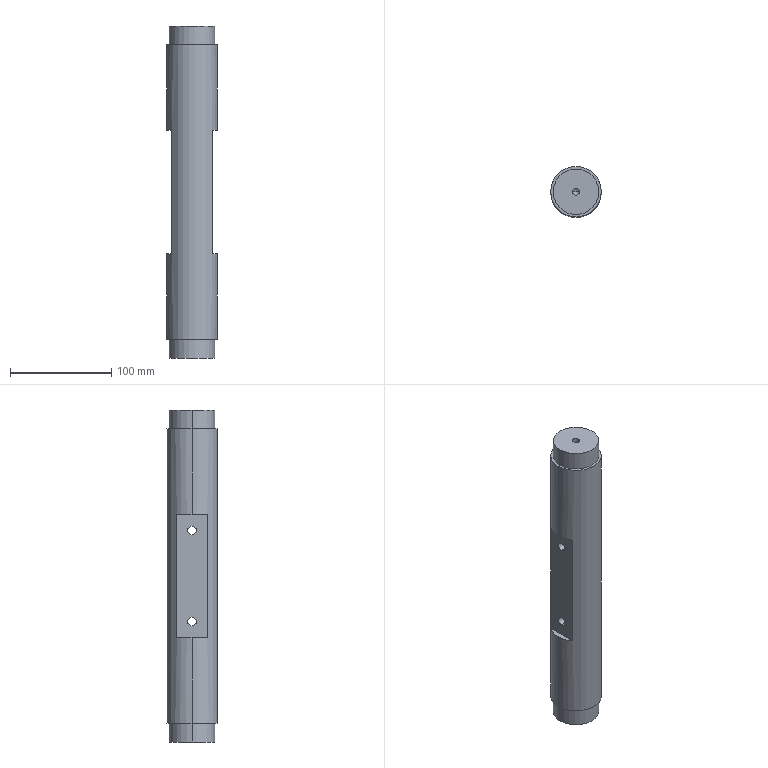Part | SolidWorks | features BaseBody 1 | 1 solid | 28 faces | box 50 x 50 x 328 mm | volume 599266 mm3 | cylinder 14 | plane 10 | cone 4 | commonest cylinder face diameters 6.8 x4 8.5 x4 45 x4 50 x2
STEP:
#1=CARTESIAN_POINT('',(-20.,0.,233.25));
#2=VERTEX_POINT('',#1);
#3=CARTESIAN_POINT('',(-20.,0.,224.75));
#4=VERTEX_POINT('',#3);
#5=CARTESIAN_POINT('',(-20.,0.,229.));
#6=DIRECTION('',(1.,0.,0.));
#7=DIRECTION('',(0.,0.,-1.));
#8=AXIS2_PLACEMENT_3D('',#5,#6,#7);
#9=CIRCLE('',#8,4.25);
#10=EDGE_CURVE('',#2,#4,#9,.T.);
#11=ORIENTED_EDGE('',*,*,#10,.F.);
#12=CARTESIAN_POINT('',(20.,0.,233.25));
#13=VERTEX_POINT('',#12);
#14=CARTESIAN_POINT('',(20.,0.,233.25));
#15=DIRECTION('',(1.,0.,0.));
#16=VECTOR('',#15,1000.);
#17=LINE('',#14,#16);
#18=EDGE_CURVE('',#2,#13,#17,.T.);
#19=ORIENTED_EDGE('',*,*,#18,.T.);
#20=CARTESIAN_POINT('',(20.,0.,224.75));
#21=VERTEX_POINT('',#20);
#22=CARTESIAN_POINT('',(20.,0.,229.));
#23=DIRECTION('',(1.,0.,0.));
#24=DIRECTION('',(0.,0.,-1.));
#25=AXIS2_PLACEMENT_3D('',#22,#23,#24);
#26=CIRCLE('',#25,4.25);
#27=EDGE_CURVE('',#13,#21,#26,.T.);
#28=ORIENTED_EDGE('',*,*,#27,.T.);
#29=CARTESIAN_POINT('',(20.,0.,224.75));
#30=DIRECTION('',(1.,0.,0.));
#31=VECTOR('',#30,1000.);
#32=LINE('',#29,#31);
#33=EDGE_CURVE('',#4,#21,#32,.T.);
#34=ORIENTED_EDGE('',*,*,#33,.F.);
#35=EDGE_LOOP('',(#11,#19,#28,#34));
#36=FACE_OUTER_BOUND('',#35,.T.);
#37=CARTESIAN_POINT('',(20.,0.,229.));
#38=DIRECTION('',(1.,0.,0.));
#39=DIRECTION('',(0.,0.,-1.));
#40=AXIS2_PLACEMENT_3D('',#37,#38,#39);
#41=CYLINDRICAL_SURFACE('',#40,4.25);
#42=ADVANCED_FACE('',(#36),#41,.F.);
#43=CARTESIAN_POINT('',(-20.,0.,143.25));
#44=VERTEX_POINT('',#43);
#45=CARTESIAN_POINT('',(-20.,0.,134.75));
#46=VERTEX_POINT('',#45);
#47=CARTESIAN_POINT('',(-20.,0.,139.));
#48=DIRECTION('',(1.,0.,0.));
#49=DIRECTION('',(0.,0.,-1.));
#50=AXIS2_PLACEMENT_3D('',#47,#48,#49);
#51=CIRCLE('',#50,4.25);
#52=EDGE_CURVE('',#44,#46,#51,.T.);
#53=ORIENTED_EDGE('',*,*,#52,.F.);
#54=CARTESIAN_POINT('',(20.,0.,143.25));
#55=VERTEX_POINT('',#54);
#56=CARTESIAN_POINT('',(20.,0.,143.25));
#57=DIRECTION('',(1.,0.,0.));
#58=VECTOR('',#57,1000.);
#59=LINE('',#56,#58);
#60=EDGE_CURVE('',#44,#55,#59,.T.);
#61=ORIENTED_EDGE('',*,*,#60,.T.);
#62=CARTESIAN_POINT('',(20.,0.,134.75));
#63=VERTEX_POINT('',#62);
#64=CARTESIAN_POINT('',(20.,0.,139.));
#65=DIRECTION('',(1.,0.,0.));
#66=DIRECTION('',(0.,0.,-1.));
#67=AXIS2_PLACEMENT_3D('',#64,#65,#66);
#68=CIRCLE('',#67,4.25);
#69=EDGE_CURVE('',#55,#63,#68,.T.);
#70=ORIENTED_EDGE('',*,*,#69,.T.);
#71=CARTESIAN_POINT('',(20.,0.,134.75));
#72=DIRECTION('',(1.,0.,0.));
#73=VECTOR('',#72,1000.);
#74=LINE('',#71,#73);
#75=EDGE_CURVE('',#46,#63,#74,.T.);
#76=ORIENTED_EDGE('',*,*,#75,.F.);
#77=EDGE_LOOP('',(#53,#61,#70,#76));
#78=FACE_OUTER_BOUND('',#77,.T.);
#79=CARTESIAN_POINT('',(20.,0.,139.));
#80=DIRECTION('',(1.,0.,0.));
#81=DIRECTION('',(0.,0.,-1.));
#82=AXIS2_PLACEMENT_3D('',#79,#80,#81);
#83=CYLINDRICAL_SURFACE('',#82,4.25);
#84=ADVANCED_FACE('',(#78),#83,.F.);
#85=CARTESIAN_POINT('',(3.4,0.,39.75));
#86=VERTEX_POINT('',#85);
#87=CARTESIAN_POINT('',(-3.4,0.,39.75));
#88=VERTEX_POINT('',#87);
#89=CARTESIAN_POINT('',(0.,0.,39.75));
#90=DIRECTION('',(0.,0.,-1.));
#91=DIRECTION('',(-1.,0.,0.));
#92=AXIS2_PLACEMENT_3D('',#89,#90,#91);
#93=CIRCLE('',#92,3.4);
#94=EDGE_CURVE('',#86,#88,#93,.T.);
#95=ORIENTED_EDGE('',*,*,#94,.F.);
#96=CARTESIAN_POINT('',(3.4,0.,20.));
#97=VERTEX_POINT('',#96);
#98=CARTESIAN_POINT('',(3.4,0.,20.));
#99=DIRECTION('',(0.,0.,-1.));
#100=VECTOR('',#99,1000.);
#101=LINE('',#98,#100);
#102=EDGE_CURVE('',#86,#97,#101,.T.);
#103=ORIENTED_EDGE('',*,*,#102,.T.);
#104=CARTESIAN_POINT('',(-3.4,0.,20.));
#105=VERTEX_POINT('',#104);
#106=CARTESIAN_POINT('',(0.,0.,20.));
#107=DIRECTION('',(0.,0.,-1.));
#108=DIRECTION('',(-1.,0.,0.));
#109=AXIS2_PLACEMENT_3D('',#106,#107,#108);
#110=CIRCLE('',#109,3.4);
#111=EDGE_CURVE('',#97,#105,#110,.T.);
#112=ORIENTED_EDGE('',*,*,#111,.T.);
#113=CARTESIAN_POINT('',(-3.4,0.,20.));
#114=DIRECTION('',(0.,0.,-1.));
#115=VECTOR('',#114,1000.);
#116=LINE('',#113,#115);
#117=EDGE_CURVE('',#88,#105,#116,.T.);
#118=ORIENTED_EDGE('',*,*,#117,.F.);
#119=EDGE_LOOP('',(#95,#103,#112,#118));
#120=FACE_OUTER_BOUND('',#119,.T.);
#121=CARTESIAN_POINT('',(0.,0.,20.));
#122=DIRECTION('',(0.,0.,-1.));
#123=DIRECTION('',(-1.,0.,0.));
#124=AXIS2_PLACEMENT_3D('',#121,#122,#123);
#125=CYLINDRICAL_SURFACE('',#124,3.4);
#126=ADVANCED_FACE('',(#120),#125,.F.);
#127=CARTESIAN_POINT('',(0.,0.,41.793));
#128=VERTEX_POINT('',#127);
#129=CARTESIAN_POINT('',(-3.4,0.,39.75));
#130=DIRECTION('',(-0.8572,0.,-0.515));
#131=VECTOR('',#130,1000.);
#132=LINE('',#129,#131);
#133=EDGE_CURVE('',#128,#88,#132,.T.);
#134=ORIENTED_EDGE('',*,*,#133,.F.);
#135=CARTESIAN_POINT('',(3.4,0.,39.75));
#136=DIRECTION('',(0.8572,0.,-0.515));
#137=VECTOR('',#136,1000.);
#138=LINE('',#135,#137);
#139=EDGE_CURVE('',#128,#86,#138,.T.);
#140=ORIENTED_EDGE('',*,*,#139,.T.);
#141=ORIENTED_EDGE('',*,*,#94,.T.);
#142=EDGE_LOOP('',(#134,#140,#141));
#143=FACE_OUTER_BOUND('',#142,.T.);
#144=CARTESIAN_POINT('',(0.,0.,39.75));
#145=DIRECTION('',(0.,0.,-1.));
#146=DIRECTION('',(-1.,0.,0.));
#147=AXIS2_PLACEMENT_3D('',#144,#145,#146);
#148=CONICAL_SURFACE('',#147,3.4,1.03);
#149=ADVANCED_FACE('',(#143),#148,.F.);
#150=CARTESIAN_POINT('',(-22.5,0.,38.5));
#151=VERTEX_POINT('',#150);
#152=CARTESIAN_POINT('',(22.5,0.,38.5));
#153=VERTEX_POINT('',#152);
#154=CARTESIAN_POINT('',(0.,0.,38.5));
#155=DIRECTION('',(0.,0.,-1.));
#156=DIRECTION('',(-1.,0.,0.));
#157=AXIS2_PLACEMENT_3D('',#154,#155,#156);
#158=CIRCLE('',#157,22.5);
#159=EDGE_CURVE('',#151,#153,#158,.T.);
#160=ORIENTED_EDGE('',*,*,#159,.T.);
#161=CARTESIAN_POINT('',(22.5,0.,20.));
#162=VERTEX_POINT('',#161);
#163=CARTESIAN_POINT('',(22.5,0.,38.5));
#164=DIRECTION('',(0.,0.,-1.));
#165=VECTOR('',#164,1000.);
#166=LINE('',#163,#165);
#167=EDGE_CURVE('',#153,#162,#166,.T.);
#168=ORIENTED_EDGE('',*,*,#167,.T.);
#169=CARTESIAN_POINT('',(-22.5,0.,20.));
#170=VERTEX_POINT('',#169);
#171=CARTESIAN_POINT('',(0.,0.,20.));
#172=DIRECTION('',(0.,0.,-1.));
#173=DIRECTION('',(-1.,0.,0.));
#174=AXIS2_PLACEMENT_3D('',#171,#172,#173);
#175=CIRCLE('',#174,22.5);
#176=EDGE_CURVE('',#170,#162,#175,.T.);
#177=ORIENTED_EDGE('',*,*,#176,.F.);
#178=CARTESIAN_POINT('',(-22.5,0.,38.5));
#179=DIRECTION('',(0.,0.,-1.));
#180=VECTOR('',#179,1000.);
#181=LINE('',#178,#180);
#182=EDGE_CURVE('',#151,#170,#181,.T.);
#183=ORIENTED_EDGE('',*,*,#182,.F.);
#184=EDGE_LOOP('',(#160,#168,#177,#183));
#185=FACE_OUTER_BOUND('',#184,.T.);
#186=CARTESIAN_POINT('',(0.,0.,38.5));
#187=DIRECTION('',(0.,0.,-1.));
#188=DIRECTION('',(-1.,0.,0.));
#189=AXIS2_PLACEMENT_3D('',#186,#187,#188);
#190=CYLINDRICAL_SURFACE('',#189,22.5);
#191=ADVANCED_FACE('',(#185),#190,.T.);
#192=CARTESIAN_POINT('',(-3.4,0.,328.25));
#193=VERTEX_POINT('',#192);
#194=CARTESIAN_POINT('',(3.4,0.,328.25));
#195=VERTEX_POINT('',#194);
#196=CARTESIAN_POINT('',(0.,0.,328.25));
#197=DIRECTION('',(0.,0.,1.));
#198=DIRECTION('',(1.,0.,0.));
#199=AXIS2_PLACEMENT_3D('',#196,#197,#198);
#200=CIRCLE('',#199,3.4);
#201=EDGE_CURVE('',#193,#195,#200,.T.);
#202=ORIENTED_EDGE('',*,*,#201,.F.);
#203=CARTESIAN_POINT('',(-3.4,0.,348.));
#204=VERTEX_POINT('',#203);
#205=CARTESIAN_POINT('',(-3.4,0.,348.));
#206=DIRECTION('',(0.,0.,1.));
#207=VECTOR('',#206,1000.);
#208=LINE('',#205,#207);
#209=EDGE_CURVE('',#193,#204,#208,.T.);
#210=ORIENTED_EDGE('',*,*,#209,.T.);
#211=CARTESIAN_POINT('',(3.4,0.,348.));
#212=VERTEX_POINT('',#211);
#213=CARTESIAN_POINT('',(0.,0.,348.));
#214=DIRECTION('',(0.,0.,1.));
#215=DIRECTION('',(1.,0.,0.));
#216=AXIS2_PLACEMENT_3D('',#213,#214,#215);
#217=CIRCLE('',#216,3.4);
#218=EDGE_CURVE('',#204,#212,#217,.T.);
#219=ORIENTED_EDGE('',*,*,#218,.T.);
#220=CARTESIAN_POINT('',(3.4,0.,348.));
#221=DIRECTION('',(0.,0.,1.));
#222=VECTOR('',#221,1000.);
#223=LINE('',#220,#222);
#224=EDGE_CURVE('',#195,#212,#223,.T.);
#225=ORIENTED_EDGE('',*,*,#224,.F.);
#226=EDGE_LOOP('',(#202,#210,#219,#225));
#227=FACE_OUTER_BOUND('',#226,.T.);
#228=CARTESIAN_POINT('',(0.,0.,348.));
#229=DIRECTION('',(0.,0.,1.));
#230=DIRECTION('',(1.,0.,0.));
#231=AXIS2_PLACEMENT_3D('',#228,#229,#230);
#232=CYLINDRICAL_SURFACE('',#231,3.4);
#233=ADVANCED_FACE('',(#227),#232,.F.);
#234=CARTESIAN_POINT('',(0.,0.,326.207));
#235=VERTEX_POINT('',#234);
#236=CARTESIAN_POINT('',(3.4,0.,328.25));
#237=DIRECTION('',(0.8572,0.,0.515));
#238=VECTOR('',#237,1000.);
#239=LINE('',#236,#238);
#240=EDGE_CURVE('',#235,#195,#239,.T.);
#241=ORIENTED_EDGE('',*,*,#240,.F.);
#242=CARTESIAN_POINT('',(-3.4,0.,328.25));
#243=DIRECTION('',(-0.8572,0.,0.515));
#244=VECTOR('',#243,1000.);
#245=LINE('',#242,#244);
#246=EDGE_CURVE('',#235,#193,#245,.T.);
#247=ORIENTED_EDGE('',*,*,#246,.T.);
#248=ORIENTED_EDGE('',*,*,#201,.T.);
#249=EDGE_LOOP('',(#241,#247,#248));
#250=FACE_OUTER_BOUND('',#249,.T.);
#251=CARTESIAN_POINT('',(0.,0.,328.25));
#252=DIRECTION('',(0.,0.,1.));
#253=DIRECTION('',(1.,0.,0.));
#254=AXIS2_PLACEMENT_3D('',#251,#252,#253);
#255=CONICAL_SURFACE('',#254,3.4,1.03);
#256=ADVANCED_FACE('',(#250),#255,.F.);
#257=CARTESIAN_POINT('',(22.5,0.,329.5));
#258=VERTEX_POINT('',#257);
#259=CARTESIAN_POINT('',(-22.5,0.,329.5));
#260=VERTEX_POINT('',#259);
#261=CARTESIAN_POINT('',(0.,0.,329.5));
#262=DIRECTION('',(0.,0.,1.));
#263=DIRECTION('',(1.,0.,0.));
#264=AXIS2_PLACEMENT_3D('',#261,#262,#263);
#265=CIRCLE('',#264,22.5);
#266=EDGE_CURVE('',#258,#260,#265,.T.);
#267=ORIENTED_EDGE('',*,*,#266,.T.);
#268=CARTESIAN_POINT('',(-22.5,0.,348.));
#269=VERTEX_POINT('',#268);
#270=CARTESIAN_POINT('',(-22.5,0.,329.5));
#271=DIRECTION('',(0.,0.,1.));
#272=VECTOR('',#271,1000.);
#273=LINE('',#270,#272);
#274=EDGE_CURVE('',#260,#269,#273,.T.);
#275=ORIENTED_EDGE('',*,*,#274,.T.);
#276=CARTESIAN_POINT('',(22.5,0.,348.));
#277=VERTEX_POINT('',#276);
#278=CARTESIAN_POINT('',(0.,0.,348.));
#279=DIRECTION('',(0.,0.,1.));
#280=DIRECTION('',(1.,0.,0.));
#281=AXIS2_PLACEMENT_3D('',#278,#279,#280);
#282=CIRCLE('',#281,22.5);
#283=EDGE_CURVE('',#277,#269,#282,.T.);
#284=ORIENTED_EDGE('',*,*,#283,.F.);
#285=CARTESIAN_POINT('',(22.5,0.,329.5));
#286=DIRECTION('',(0.,0.,1.));
#287=VECTOR('',#286,1000.);
#288=LINE('',#285,#287);
#289=EDGE_CURVE('',#258,#277,#288,.T.);
#290=ORIENTED_EDGE('',*,*,#289,.F.);
#291=EDGE_LOOP('',(#267,#275,#284,#290));
#292=FACE_OUTER_BOUND('',#291,.T.);
#293=CARTESIAN_POINT('',(0.,0.,329.5));
#294=DIRECTION('',(0.,0.,1.));
#295=DIRECTION('',(1.,0.,0.));
#296=AXIS2_PLACEMENT_3D('',#293,#294,#295);
#297=CYLINDRICAL_SURFACE('',#296,22.5);
#298=ADVANCED_FACE('',(#292),#297,.T.);
#299=CARTESIAN_POINT('',(25.,0.,329.5));
#300=VERTEX_POINT('',#299);
#301=CARTESIAN_POINT('',(-25.,0.,329.5));
#302=VERTEX_POINT('',#301);
#303=CARTESIAN_POINT('',(0.,0.,329.5));
#304=DIRECTION('',(0.,0.,1.));
#305=DIRECTION('',(1.,0.,0.));
#306=AXIS2_PLACEMENT_3D('',#303,#304,#305);
#307=CIRCLE('',#306,25.);
#308=EDGE_CURVE('',#300,#302,#307,.T.);
#309=ORIENTED_EDGE('',*,*,#308,.F.);
#310=CARTESIAN_POINT('',(25.,0.,245.));
#311=VERTEX_POINT('',#310);
#312=CARTESIAN_POINT('',(25.,0.,368.));
#313=DIRECTION('',(0.,0.,-1.));
#314=VECTOR('',#313,1000.);
#315=LINE('',#312,#314);
#316=EDGE_CURVE('',#300,#311,#315,.T.);
#317=ORIENTED_EDGE('',*,*,#316,.T.);
#318=CARTESIAN_POINT('',(20.,15.,245.));
#319=VERTEX_POINT('',#318);
#320=CARTESIAN_POINT('',(0.,0.,245.));
#321=DIRECTION('',(0.,0.,1.));
#322=DIRECTION('',(1.,0.,0.));
#323=AXIS2_PLACEMENT_3D('',#320,#321,#322);
#324=CIRCLE('',#323,25.);
#325=EDGE_CURVE('',#311,#319,#324,.T.);
#326=ORIENTED_EDGE('',*,*,#325,.T.);
#327=CARTESIAN_POINT('',(20.,15.,123.));
#328=VERTEX_POINT('',#327);
#329=CARTESIAN_POINT('',(20.,15.,368.));
#330=DIRECTION('',(0.,0.,-1.));
#331=VECTOR('',#330,1000.);
#332=LINE('',#329,#331);
#333=EDGE_CURVE('',#319,#328,#332,.T.);
#334=ORIENTED_EDGE('',*,*,#333,.T.);
#335=CARTESIAN_POINT('',(25.,0.,123.));
#336=VERTEX_POINT('',#335);
#337=CARTESIAN_POINT('',(0.,0.,123.));
#338=DIRECTION('',(0.,0.,-1.));
#339=DIRECTION('',(-1.,0.,0.));
#340=AXIS2_PLACEMENT_3D('',#337,#338,#339);
#341=CIRCLE('',#340,25.);
#342=EDGE_CURVE('',#328,#336,#341,.T.);
#343=ORIENTED_EDGE('',*,*,#342,.T.);
#344=CARTESIAN_POINT('',(25.,0.,38.5));
#345=VERTEX_POINT('',#344);
#346=CARTESIAN_POINT('',(25.,0.,368.));
#347=DIRECTION('',(0.,0.,-1.));
#348=VECTOR('',#347,1000.);
#349=LINE('',#346,#348);
#350=EDGE_CURVE('',#336,#345,#349,.T.);
#351=ORIENTED_EDGE('',*,*,#350,.T.);
#352=CARTESIAN_POINT('',(-25.,0.,38.5));
#353=VERTEX_POINT('',#352);
#354=CARTESIAN_POINT('',(0.,0.,38.5));
#355=DIRECTION('',(0.,0.,-1.));
#356=DIRECTION('',(-1.,0.,0.));
#357=AXIS2_PLACEMENT_3D('',#354,#355,#356);
#358=CIRCLE('',#357,25.);
#359=EDGE_CURVE('',#353,#345,#358,.T.);
#360=ORIENTED_EDGE('',*,*,#359,.F.);
#361=CARTESIAN_POINT('',(-25.,0.,123.));
#362=VERTEX_POINT('',#361);
#363=CARTESIAN_POINT('',(-25.,0.,368.));
#364=DIRECTION('',(0.,0.,-1.));
#365=VECTOR('',#364,1000.);
#366=LINE('',#363,#365);
#367=EDGE_CURVE('',#362,#353,#366,.T.);
#368=ORIENTED_EDGE('',*,*,#367,.F.);
#369=CARTESIAN_POINT('',(-20.,15.,123.));
#370=VERTEX_POINT('',#369);
#371=CARTESIAN_POINT('',(0.,0.,123.));
#372=DIRECTION('',(0.,0.,-1.));
#373=DIRECTION('',(-1.,0.,0.));
#374=AXIS2_PLACEMENT_3D('',#371,#372,#373);
#375=CIRCLE('',#374,25.);
#376=EDGE_CURVE('',#362,#370,#375,.T.);
#377=ORIENTED_EDGE('',*,*,#376,.T.);
#378=CARTESIAN_POINT('',(-20.,15.,245.));
#379=VERTEX_POINT('',#378);
#380=CARTESIAN_POINT('',(-20.,15.,368.));
#381=DIRECTION('',(0.,0.,1.));
#382=VECTOR('',#381,1000.);
#383=LINE('',#380,#382);
#384=EDGE_CURVE('',#370,#379,#383,.T.);
#385=ORIENTED_EDGE('',*,*,#384,.T.);
#386=CARTESIAN_POINT('',(-25.,0.,245.));
#387=VERTEX_POINT('',#386);
#388=CARTESIAN_POINT('',(0.,0.,245.));
#389=DIRECTION('',(0.,0.,1.));
#390=DIRECTION('',(1.,0.,0.));
#391=AXIS2_PLACEMENT_3D('',#388,#389,#390);
#392=CIRCLE('',#391,25.);
#393=EDGE_CURVE('',#379,#387,#392,.T.);
#394=ORIENTED_EDGE('',*,*,#393,.T.);
#395=CARTESIAN_POINT('',(-25.,0.,368.));
#396=DIRECTION('',(0.,0.,-1.));
#397=VECTOR('',#396,1000.);
#398=LINE('',#395,#397);
#399=EDGE_CURVE('',#302,#387,#398,.T.);
#400=ORIENTED_EDGE('',*,*,#399,.F.);
#401=EDGE_LOOP('',(#309,#317,#326,#334,#343,#351,#360,#368,#377,#385,#394,#400));
#402=FACE_OUTER_BOUND('',#401,.T.);
#403=CARTESIAN_POINT('',(0.,0.,368.));
#404=DIRECTION('',(0.,0.,-1.));
#405=DIRECTION('',(-1.,0.,0.));
#406=AXIS2_PLACEMENT_3D('',#403,#404,#405);
#407=CYLINDRICAL_SURFACE('',#406,25.);
#408=ADVANCED_FACE('',(#402),#407,.T.);
#409=CARTESIAN_POINT('',(20.,0.,229.));
#410=DIRECTION('',(1.,0.,0.));
#411=DIRECTION('',(0.,0.,-1.));
#412=AXIS2_PLACEMENT_3D('',#409,#410,#411);
#413=CIRCLE('',#412,4.25);
#414=EDGE_CURVE('',#21,#13,#413,.T.);
#415=ORIENTED_EDGE('',*,*,#414,.F.);
#416=ORIENTED_EDGE('',*,*,#27,.F.);
#417=EDGE_LOOP('',(#415,#416));
#418=FACE_BOUND('',#417,.T.);
#419=CARTESIAN_POINT('',(20.,-15.,245.));
#420=VERTEX_POINT('',#419);
#421=CARTESIAN_POINT('',(20.,-250.,245.));
#422=DIRECTION('',(0.,1.,0.));
#423=VECTOR('',#422,1000.);
#424=LINE('',#421,#423);
#425=EDGE_CURVE('',#420,#319,#424,.T.);
#426=ORIENTED_EDGE('',*,*,#425,.F.);
#427=CARTESIAN_POINT('',(20.,-15.,123.));
#428=VERTEX_POINT('',#427);
#429=CARTESIAN_POINT('',(20.,-15.,368.));
#430=DIRECTION('',(0.,0.,1.));
#431=VECTOR('',#430,1000.);
#432=LINE('',#429,#431);
#433=EDGE_CURVE('',#428,#420,#432,.T.);
#434=ORIENTED_EDGE('',*,*,#433,.F.);
#435=CARTESIAN_POINT('',(20.,-250.,123.));
#436=DIRECTION('',(0.,1.,0.));
#437=VECTOR('',#436,1000.);
#438=LINE('',#435,#437);
#439=EDGE_CURVE('',#428,#328,#438,.T.);
#440=ORIENTED_EDGE('',*,*,#439,.T.);
#441=ORIENTED_EDGE('',*,*,#333,.F.);
#442=EDGE_LOOP('',(#426,#434,#440,#441));
#443=FACE_OUTER_BOUND('',#442,.T.);
#444=CARTESIAN_POINT('',(20.,0.,139.));
#445=DIRECTION('',(1.,0.,0.));
#446=DIRECTION('',(0.,0.,-1.));
#447=AXIS2_PLACEMENT_3D('',#444,#445,#446);
#448=CIRCLE('',#447,4.25);
#449=EDGE_CURVE('',#63,#55,#448,.T.);
#450=ORIENTED_EDGE('',*,*,#449,.F.);
#451=ORIENTED_EDGE('',*,*,#69,.F.);
#452=EDGE_LOOP('',(#450,#451));
#453=FACE_BOUND('',#452,.T.);
#454=CARTESIAN_POINT('',(20.,-250.,123.));
#455=DIRECTION('',(-1.,0.,0.));
#456=DIRECTION('',(0.,0.,1.));
#457=AXIS2_PLACEMENT_3D('',#454,#455,#456);
#458=PLANE('',#457);
#459=ADVANCED_FACE('',(#418,#443,#453),#458,.F.);
#460=ORIENTED_EDGE('',*,*,#316,.F.);
#461=CARTESIAN_POINT('',(0.,0.,329.5));
#462=DIRECTION('',(0.,0.,1.));
#463=DIRECTION('',(1.,0.,0.));
#464=AXIS2_PLACEMENT_3D('',#461,#462,#463);
#465=CIRCLE('',#464,25.);
#466=EDGE_CURVE('',#302,#300,#465,.T.);
#467=ORIENTED_EDGE('',*,*,#466,.F.);
#468=ORIENTED_EDGE('',*,*,#399,.T.);
#469=CARTESIAN_POINT('',(-20.,-15.,245.));
#470=VERTEX_POINT('',#469);
#471=CARTESIAN_POINT('',(0.,0.,245.));
#472=DIRECTION('',(0.,0.,1.));
#473=DIRECTION('',(1.,0.,0.));
#474=AXIS2_PLACEMENT_3D('',#471,#472,#473);
#475=CIRCLE('',#474,25.);
#476=EDGE_CURVE('',#387,#470,#475,.T.);
#477=ORIENTED_EDGE('',*,*,#476,.T.);
#478=CARTESIAN_POINT('',(-20.,-15.,123.));
#479=VERTEX_POINT('',#478);
#480=CARTESIAN_POINT('',(-20.,-15.,368.));
#481=DIRECTION('',(0.,0.,-1.));
#482=VECTOR('',#481,1000.);
#483=LINE('',#480,#482);
#484=EDGE_CURVE('',#470,#479,#483,.T.);
#485=ORIENTED_EDGE('',*,*,#484,.T.);
#486=CARTESIAN_POINT('',(0.,0.,123.));
#487=DIRECTION('',(0.,0.,-1.));
#488=DIRECTION('',(-1.,0.,0.));
#489=AXIS2_PLACEMENT_3D('',#486,#487,#488);
#490=CIRCLE('',#489,25.);
#491=EDGE_CURVE('',#479,#362,#490,.T.);
#492=ORIENTED_EDGE('',*,*,#491,.T.);
#493=ORIENTED_EDGE('',*,*,#367,.T.);
#494=CARTESIAN_POINT('',(0.,0.,38.5));
#495=DIRECTION('',(0.,0.,-1.));
#496=DIRECTION('',(-1.,0.,0.));
#497=AXIS2_PLACEMENT_3D('',#494,#495,#496);
#498=CIRCLE('',#497,25.);
#499=EDGE_CURVE('',#345,#353,#498,.T.);
#500=ORIENTED_EDGE('',*,*,#499,.F.);
#501=ORIENTED_EDGE('',*,*,#350,.F.);
#502=CARTESIAN_POINT('',(0.,0.,123.));
#503=DIRECTION('',(0.,0.,-1.));
#504=DIRECTION('',(-1.,0.,0.));
#505=AXIS2_PLACEMENT_3D('',#502,#503,#504);
#506=CIRCLE('',#505,25.);
#507=EDGE_CURVE('',#336,#428,#506,.T.);
#508=ORIENTED_EDGE('',*,*,#507,.T.);
#509=ORIENTED_EDGE('',*,*,#433,.T.);
#510=CARTESIAN_POINT('',(0.,0.,245.));
#511=DIRECTION('',(0.,0.,1.));
#512=DIRECTION('',(1.,0.,0.));
#513=AXIS2_PLACEMENT_3D('',#510,#511,#512);
#514=CIRCLE('',#513,25.);
#515=EDGE_CURVE('',#420,#311,#514,.T.);
#516=ORIENTED_EDGE('',*,*,#515,.T.);
#517=EDGE_LOOP('',(#460,#467,#468,#477,#485,#492,#493,#500,#501,#508,#509,#516));
#518=FACE_OUTER_BOUND('',#517,.T.);
#519=CARTESIAN_POINT('',(0.,0.,368.));
#520=DIRECTION('',(0.,0.,-1.));
#521=DIRECTION('',(-1.,0.,0.));
#522=AXIS2_PLACEMENT_3D('',#519,#520,#521);
#523=CYLINDRICAL_SURFACE('',#522,25.);
#524=ADVANCED_FACE('',(#518),#523,.T.);
#525=ORIENTED_EDGE('',*,*,#439,.F.);
#526=ORIENTED_EDGE('',*,*,#507,.F.);
#527=ORIENTED_EDGE('',*,*,#342,.F.);
#528=EDGE_LOOP('',(#525,#526,#527));
#529=FACE_OUTER_BOUND('',#528,.T.);
#530=CARTESIAN_POINT('',(20.,-250.,123.));
#531=DIRECTION('',(0.,0.,-1.));
#532=DIRECTION('',(-1.,0.,0.));
#533=AXIS2_PLACEMENT_3D('',#530,#531,#532);
#534=PLANE('',#533);
#535=ADVANCED_FACE('',(#529),#534,.F.);
#536=ORIENTED_EDGE('',*,*,#425,.T.);
#537=ORIENTED_EDGE('',*,*,#325,.F.);
#538=ORIENTED_EDGE('',*,*,#515,.F.);
#539=EDGE_LOOP('',(#536,#537,#538));
#540=FACE_OUTER_BOUND('',#539,.T.);
#541=CARTESIAN_POINT('',(20.,-250.,245.));
#542=DIRECTION('',(0.,0.,1.));
#543=DIRECTION('',(1.,0.,0.));
#544=AXIS2_PLACEMENT_3D('',#541,#542,#543);
#545=PLANE('',#544);
#546=ADVANCED_FACE('',(#540),#545,.F.);
#547=CARTESIAN_POINT('',(-20.,-250.,123.));
#548=DIRECTION('',(0.,1.,0.));
#549=VECTOR('',#548,1000.);
#550=LINE('',#547,#549);
#551=EDGE_CURVE('',#479,#370,#550,.T.);
#552=ORIENTED_EDGE('',*,*,#551,.T.);
#553=ORIENTED_EDGE('',*,*,#376,.F.);
#554=ORIENTED_EDGE('',*,*,#491,.F.);
#555=EDGE_LOOP('',(#552,#553,#554));
#556=FACE_OUTER_BOUND('',#555,.T.);
#557=CARTESIAN_POINT('',(-53.509,-250.,123.));
#558=DIRECTION('',(0.,0.,-1.));
#559=DIRECTION('',(-1.,0.,0.));
#560=AXIS2_PLACEMENT_3D('',#557,#558,#559);
#561=PLANE('',#560);
#562=ADVANCED_FACE('',(#556),#561,.F.);
#563=CARTESIAN_POINT('',(-20.,0.,229.));
#564=DIRECTION('',(1.,0.,0.));
#565=DIRECTION('',(0.,0.,-1.));
#566=AXIS2_PLACEMENT_3D('',#563,#564,#565);
#567=CIRCLE('',#566,4.25);
#568=EDGE_CURVE('',#4,#2,#567,.T.);
#569=ORIENTED_EDGE('',*,*,#568,.T.);
#570=ORIENTED_EDGE('',*,*,#10,.T.);
#571=EDGE_LOOP('',(#569,#570));
#572=FACE_BOUND('',#571,.T.);
#573=CARTESIAN_POINT('',(-20.,0.,139.));
#574=DIRECTION('',(1.,0.,0.));
#575=DIRECTION('',(0.,0.,-1.));
#576=AXIS2_PLACEMENT_3D('',#573,#574,#575);
#577=CIRCLE('',#576,4.25);
#578=EDGE_CURVE('',#46,#44,#577,.T.);
#579=ORIENTED_EDGE('',*,*,#578,.T.);
#580=ORIENTED_EDGE('',*,*,#52,.T.);
#581=EDGE_LOOP('',(#579,#580));
#582=FACE_BOUND('',#581,.T.);
#583=CARTESIAN_POINT('',(-20.,-250.,245.));
#584=DIRECTION('',(0.,1.,0.));
#585=VECTOR('',#584,1000.);
#586=LINE('',#583,#585);
#587=EDGE_CURVE('',#470,#379,#586,.T.);
#588=ORIENTED_EDGE('',*,*,#587,.T.);
#589=ORIENTED_EDGE('',*,*,#384,.F.);
#590=ORIENTED_EDGE('',*,*,#551,.F.);
#591=ORIENTED_EDGE('',*,*,#484,.F.);
#592=EDGE_LOOP('',(#588,#589,#590,#591));
#593=FACE_OUTER_BOUND('',#592,.T.);
#594=CARTESIAN_POINT('',(-20.,-250.,123.));
#595=DIRECTION('',(1.,0.,0.));
#596=DIRECTION('',(0.,0.,-1.));
#597=AXIS2_PLACEMENT_3D('',#594,#595,#596);
#598=PLANE('',#597);
#599=ADVANCED_FACE('',(#572,#582,#593),#598,.F.);
#600=ORIENTED_EDGE('',*,*,#587,.F.);
#601=ORIENTED_EDGE('',*,*,#476,.F.);
#602=ORIENTED_EDGE('',*,*,#393,.F.);
#603=EDGE_LOOP('',(#600,#601,#602));
#604=FACE_OUTER_BOUND('',#603,.T.);
#605=CARTESIAN_POINT('',(-53.509,-250.,245.));
#606=DIRECTION('',(0.,0.,1.));
#607=DIRECTION('',(1.,0.,0.));
#608=AXIS2_PLACEMENT_3D('',#605,#606,#607);
#609=PLANE('',#608);
#610=ADVANCED_FACE('',(#604),#609,.F.);
#611=ORIENTED_EDGE('',*,*,#266,.F.);
#612=CARTESIAN_POINT('',(0.,0.,329.5));
#613=DIRECTION('',(0.,0.,1.));
#614=DIRECTION('',(1.,0.,0.));
#615=AXIS2_PLACEMENT_3D('',#612,#613,#614);
#616=CIRCLE('',#615,22.5);
#617=EDGE_CURVE('',#260,#258,#616,.T.);
#618=ORIENTED_EDGE('',*,*,#617,.F.);
#619=EDGE_LOOP('',(#611,#618));
#620=FACE_BOUND('',#619,.T.);
#621=ORIENTED_EDGE('',*,*,#466,.T.);
#622=ORIENTED_EDGE('',*,*,#308,.T.);
#623=EDGE_LOOP('',(#621,#622));
#624=FACE_OUTER_BOUND('',#623,.T.);
#625=CARTESIAN_POINT('',(0.,0.,329.5));
#626=DIRECTION('',(0.,0.,1.));
#627=DIRECTION('',(1.,0.,0.));
#628=AXIS2_PLACEMENT_3D('',#625,#626,#627);
#629=PLANE('',#628);
#630=ADVANCED_FACE('',(#620,#624),#629,.T.);
#631=ORIENTED_EDGE('',*,*,#274,.F.);
#632=ORIENTED_EDGE('',*,*,#617,.T.);
#633=ORIENTED_EDGE('',*,*,#289,.T.);
#634=CARTESIAN_POINT('',(0.,0.,348.));
#635=DIRECTION('',(0.,0.,1.));
#636=DIRECTION('',(1.,0.,0.));
#637=AXIS2_PLACEMENT_3D('',#634,#635,#636);
#638=CIRCLE('',#637,22.5);
#639=EDGE_CURVE('',#269,#277,#638,.T.);
#640=ORIENTED_EDGE('',*,*,#639,.F.);
#641=EDGE_LOOP('',(#631,#632,#633,#640));
#642=FACE_OUTER_BOUND('',#641,.T.);
#643=CARTESIAN_POINT('',(0.,0.,329.5));
#644=DIRECTION('',(0.,0.,1.));
#645=DIRECTION('',(1.,0.,0.));
#646=AXIS2_PLACEMENT_3D('',#643,#644,#645);
#647=CYLINDRICAL_SURFACE('',#646,22.5);
#648=ADVANCED_FACE('',(#642),#647,.T.);
#649=ORIENTED_EDGE('',*,*,#246,.F.);
#650=ORIENTED_EDGE('',*,*,#240,.T.);
#651=CARTESIAN_POINT('',(0.,0.,328.25));
#652=DIRECTION('',(0.,0.,1.));
#653=DIRECTION('',(1.,0.,0.));
#654=AXIS2_PLACEMENT_3D('',#651,#652,#653);
#655=CIRCLE('',#654,3.4);
#656=EDGE_CURVE('',#195,#193,#655,.T.);
#657=ORIENTED_EDGE('',*,*,#656,.T.);
#658=EDGE_LOOP('',(#649,#650,#657));
#659=FACE_OUTER_BOUND('',#658,.T.);
#660=CARTESIAN_POINT('',(0.,0.,328.25));
#661=DIRECTION('',(0.,0.,1.));
#662=DIRECTION('',(1.,0.,0.));
#663=AXIS2_PLACEMENT_3D('',#660,#661,#662);
#664=CONICAL_SURFACE('',#663,3.4,1.03);
#665=ADVANCED_FACE('',(#659),#664,.F.);
#666=ORIENTED_EDGE('',*,*,#209,.F.);
#667=ORIENTED_EDGE('',*,*,#656,.F.);
#668=ORIENTED_EDGE('',*,*,#224,.T.);
#669=CARTESIAN_POINT('',(0.,0.,348.));
#670=DIRECTION('',(0.,0.,1.));
#671=DIRECTION('',(1.,0.,0.));
#672=AXIS2_PLACEMENT_3D('',#669,#670,#671);
#673=CIRCLE('',#672,3.4);
#674=EDGE_CURVE('',#212,#204,#673,.T.);
#675=ORIENTED_EDGE('',*,*,#674,.T.);
#676=EDGE_LOOP('',(#666,#667,#668,#675));
#677=FACE_OUTER_BOUND('',#676,.T.);
#678=CARTESIAN_POINT('',(0.,0.,348.));
#679=DIRECTION('',(0.,0.,1.));
#680=DIRECTION('',(1.,0.,0.));
#681=AXIS2_PLACEMENT_3D('',#678,#679,#680);
#682=CYLINDRICAL_SURFACE('',#681,3.4);
#683=ADVANCED_FACE('',(#677),#682,.F.);
#684=ORIENTED_EDGE('',*,*,#674,.F.);
#685=ORIENTED_EDGE('',*,*,#218,.F.);
#686=EDGE_LOOP('',(#684,#685));
#687=FACE_BOUND('',#686,.T.);
#688=ORIENTED_EDGE('',*,*,#283,.T.);
#689=ORIENTED_EDGE('',*,*,#639,.T.);
#690=EDGE_LOOP('',(#688,#689));
#691=FACE_OUTER_BOUND('',#690,.T.);
#692=CARTESIAN_POINT('',(0.,0.,348.));
#693=DIRECTION('',(0.,0.,1.));
#694=DIRECTION('',(1.,0.,0.));
#695=AXIS2_PLACEMENT_3D('',#692,#693,#694);
#696=PLANE('',#695);
#697=ADVANCED_FACE('',(#687,#691),#696,.T.);
#698=ORIENTED_EDGE('',*,*,#159,.F.);
#699=CARTESIAN_POINT('',(0.,0.,38.5));
#700=DIRECTION('',(0.,0.,-1.));
#701=DIRECTION('',(-1.,0.,0.));
#702=AXIS2_PLACEMENT_3D('',#699,#700,#701);
#703=CIRCLE('',#702,22.5);
#704=EDGE_CURVE('',#153,#151,#703,.T.);
#705=ORIENTED_EDGE('',*,*,#704,.F.);
#706=EDGE_LOOP('',(#698,#705));
#707=FACE_BOUND('',#706,.T.);
#708=ORIENTED_EDGE('',*,*,#359,.T.);
#709=ORIENTED_EDGE('',*,*,#499,.T.);
#710=EDGE_LOOP('',(#708,#709));
#711=FACE_OUTER_BOUND('',#710,.T.);
#712=CARTESIAN_POINT('',(0.,0.,38.5));
#713=DIRECTION('',(0.,0.,-1.));
#714=DIRECTION('',(-1.,0.,0.));
#715=AXIS2_PLACEMENT_3D('',#712,#713,#714);
#716=PLANE('',#715);
#717=ADVANCED_FACE('',(#707,#711),#716,.T.);
#718=ORIENTED_EDGE('',*,*,#167,.F.);
#719=ORIENTED_EDGE('',*,*,#704,.T.);
#720=ORIENTED_EDGE('',*,*,#182,.T.);
#721=CARTESIAN_POINT('',(0.,0.,20.));
#722=DIRECTION('',(0.,0.,-1.));
#723=DIRECTION('',(-1.,0.,0.));
#724=AXIS2_PLACEMENT_3D('',#721,#722,#723);
#725=CIRCLE('',#724,22.5);
#726=EDGE_CURVE('',#162,#170,#725,.T.);
#727=ORIENTED_EDGE('',*,*,#726,.F.);
#728=EDGE_LOOP('',(#718,#719,#720,#727));
#729=FACE_OUTER_BOUND('',#728,.T.);
#730=CARTESIAN_POINT('',(0.,0.,38.5));
#731=DIRECTION('',(0.,0.,-1.));
#732=DIRECTION('',(-1.,0.,0.));
#733=AXIS2_PLACEMENT_3D('',#730,#731,#732);
#734=CYLINDRICAL_SURFACE('',#733,22.5);
#735=ADVANCED_FACE('',(#729),#734,.T.);
#736=ORIENTED_EDGE('',*,*,#139,.F.);
#737=ORIENTED_EDGE('',*,*,#133,.T.);
#738=CARTESIAN_POINT('',(0.,0.,39.75));
#739=DIRECTION('',(0.,0.,-1.));
#740=DIRECTION('',(-1.,0.,0.));
#741=AXIS2_PLACEMENT_3D('',#738,#739,#740);
#742=CIRCLE('',#741,3.4);
#743=EDGE_CURVE('',#88,#86,#742,.T.);
#744=ORIENTED_EDGE('',*,*,#743,.T.);
#745=EDGE_LOOP('',(#736,#737,#744));
#746=FACE_OUTER_BOUND('',#745,.T.);
#747=CARTESIAN_POINT('',(0.,0.,39.75));
#748=DIRECTION('',(0.,0.,-1.));
#749=DIRECTION('',(-1.,0.,0.));
#750=AXIS2_PLACEMENT_3D('',#747,#748,#749);
#751=CONICAL_SURFACE('',#750,3.4,1.03);
#752=ADVANCED_FACE('',(#746),#751,.F.);
#753=ORIENTED_EDGE('',*,*,#102,.F.);
#754=ORIENTED_EDGE('',*,*,#743,.F.);
#755=ORIENTED_EDGE('',*,*,#117,.T.);
#756=CARTESIAN_POINT('',(0.,0.,20.));
#757=DIRECTION('',(0.,0.,-1.));
#758=DIRECTION('',(-1.,0.,0.));
#759=AXIS2_PLACEMENT_3D('',#756,#757,#758);
#760=CIRCLE('',#759,3.4);
#761=EDGE_CURVE('',#105,#97,#760,.T.);
#762=ORIENTED_EDGE('',*,*,#761,.T.);
#763=EDGE_LOOP('',(#753,#754,#755,#762));
#764=FACE_OUTER_BOUND('',#763,.T.);
#765=CARTESIAN_POINT('',(0.,0.,20.));
#766=DIRECTION('',(0.,0.,-1.));
#767=DIRECTION('',(-1.,0.,0.));
#768=AXIS2_PLACEMENT_3D('',#765,#766,#767);
#769=CYLINDRICAL_SURFACE('',#768,3.4);
#770=ADVANCED_FACE('',(#764),#769,.F.);
#771=ORIENTED_EDGE('',*,*,#761,.F.);
#772=ORIENTED_EDGE('',*,*,#111,.F.);
#773=EDGE_LOOP('',(#771,#772));
#774=FACE_BOUND('',#773,.T.);
#775=ORIENTED_EDGE('',*,*,#176,.T.);
#776=ORIENTED_EDGE('',*,*,#726,.T.);
#777=EDGE_LOOP('',(#775,#776));
#778=FACE_OUTER_BOUND('',#777,.T.);
#779=CARTESIAN_POINT('',(0.,0.,20.));
#780=DIRECTION('',(0.,0.,1.));
#781=DIRECTION('',(1.,0.,0.));
#782=AXIS2_PLACEMENT_3D('',#779,#780,#781);
#783=PLANE('',#782);
#784=ADVANCED_FACE('',(#774,#778),#783,.F.);
#785=ORIENTED_EDGE('',*,*,#60,.F.);
#786=ORIENTED_EDGE('',*,*,#578,.F.);
#787=ORIENTED_EDGE('',*,*,#75,.T.);
#788=ORIENTED_EDGE('',*,*,#449,.T.);
#789=EDGE_LOOP('',(#785,#786,#787,#788));
#790=FACE_OUTER_BOUND('',#789,.T.);
#791=CARTESIAN_POINT('',(20.,0.,139.));
#792=DIRECTION('',(1.,0.,0.));
#793=DIRECTION('',(0.,0.,-1.));
#794=AXIS2_PLACEMENT_3D('',#791,#792,#793);
#795=CYLINDRICAL_SURFACE('',#794,4.25);
#796=ADVANCED_FACE('',(#790),#795,.F.);
#797=ORIENTED_EDGE('',*,*,#18,.F.);
#798=ORIENTED_EDGE('',*,*,#568,.F.);
#799=ORIENTED_EDGE('',*,*,#33,.T.);
#800=ORIENTED_EDGE('',*,*,#414,.T.);
#801=EDGE_LOOP('',(#797,#798,#799,#800));
#802=FACE_OUTER_BOUND('',#801,.T.);
#803=CARTESIAN_POINT('',(20.,0.,229.));
#804=DIRECTION('',(1.,0.,0.));
#805=DIRECTION('',(0.,0.,-1.));
#806=AXIS2_PLACEMENT_3D('',#803,#804,#805);
#807=CYLINDRICAL_SURFACE('',#806,4.25);
#808=ADVANCED_FACE('',(#802),#807,.F.);
#809=CLOSED_SHELL('',(#42,#84,#126,#149,#191,#233,#256,#298,#408,#459,#524,#535,#546,#562,#599,#610,#630,#648,#665,#683,#697,#717,#735,#752,#770,#784,#796,#808));
#810=MANIFOLD_SOLID_BREP('',#809);
#811=CARTESIAN_POINT('',(0.,0.,0.));
#812=DIRECTION('',(0.,0.,1.));
#813=DIRECTION('',(1.,0.,0.));
#814=AXIS2_PLACEMENT_3D('',#811,#812,#813);
#815=(LENGTH_UNIT()NAMED_UNIT(*)SI_UNIT(.MILLI.,.METRE.));
#816=UNCERTAINTY_MEASURE_WITH_UNIT(LENGTH_MEASURE(0.00001),#815,'','');
#817=(NAMED_UNIT(*)PLANE_ANGLE_UNIT()SI_UNIT($,.RADIAN.));
#818=(NAMED_UNIT(*)SI_UNIT($,.STERADIAN.)SOLID_ANGLE_UNIT());
#819=(GEOMETRIC_REPRESENTATION_CONTEXT(3)GLOBAL_UNCERTAINTY_ASSIGNED_CONTEXT((#816))GLOBAL_UNIT_ASSIGNED_CONTEXT((#815,#817,#818))REPRESENTATION_CONTEXT('',''));
#820=ADVANCED_BREP_SHAPE_REPRESENTATION('',(#810,#814),#819);